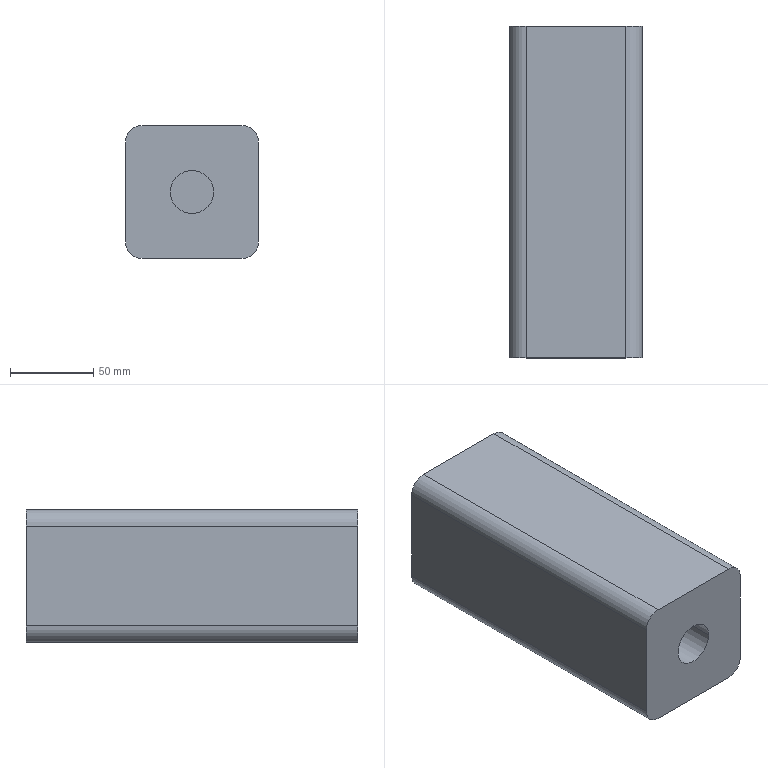Part | SolidWorks | features HoleWzd 2, Extrusion 1, Fillet 1, ICE 1 | 1 solid | 29 faces | box 80 x 199.7 x 80 mm | volume 1203112 mm3 | cylinder 14 | cone 8 | plane 7 | commonest cylinder face diameters 8.5 x8 20 x4 26 x2
STEP:
#1=CARTESIAN_POINT('',(20.,139.7,14.25));
#2=VERTEX_POINT('',#1);
#3=CARTESIAN_POINT('',(20.,139.7,5.75));
#4=VERTEX_POINT('',#3);
#5=CARTESIAN_POINT('',(20.,139.7,10.));
#6=DIRECTION('',(1.,0.,0.));
#7=DIRECTION('',(0.,0.,-1.));
#8=AXIS2_PLACEMENT_3D('',#5,#6,#7);
#9=CIRCLE('',#8,4.25);
#10=EDGE_CURVE('',#2,#4,#9,.T.);
#11=ORIENTED_EDGE('',*,*,#10,.F.);
#12=CARTESIAN_POINT('',(40.,139.7,14.25));
#13=VERTEX_POINT('',#12);
#14=CARTESIAN_POINT('',(40.,139.7,14.25));
#15=DIRECTION('',(1.,0.,0.));
#16=VECTOR('',#15,1000.);
#17=LINE('',#14,#16);
#18=EDGE_CURVE('',#2,#13,#17,.T.);
#19=ORIENTED_EDGE('',*,*,#18,.T.);
#20=CARTESIAN_POINT('',(40.,139.7,5.75));
#21=VERTEX_POINT('',#20);
#22=CARTESIAN_POINT('',(40.,139.7,10.));
#23=DIRECTION('',(1.,0.,0.));
#24=DIRECTION('',(0.,0.,-1.));
#25=AXIS2_PLACEMENT_3D('',#22,#23,#24);
#26=CIRCLE('',#25,4.25);
#27=EDGE_CURVE('',#13,#21,#26,.T.);
#28=ORIENTED_EDGE('',*,*,#27,.T.);
#29=CARTESIAN_POINT('',(40.,139.7,5.75));
#30=DIRECTION('',(1.,0.,0.));
#31=VECTOR('',#30,1000.);
#32=LINE('',#29,#31);
#33=EDGE_CURVE('',#4,#21,#32,.T.);
#34=ORIENTED_EDGE('',*,*,#33,.F.);
#35=EDGE_LOOP('',(#11,#19,#28,#34));
#36=FACE_OUTER_BOUND('',#35,.T.);
#37=CARTESIAN_POINT('',(40.,139.7,10.));
#38=DIRECTION('',(1.,0.,0.));
#39=DIRECTION('',(0.,0.,-1.));
#40=AXIS2_PLACEMENT_3D('',#37,#38,#39);
#41=CYLINDRICAL_SURFACE('',#40,4.25);
#42=ADVANCED_FACE('',(#36),#41,.F.);
#43=CARTESIAN_POINT('',(17.446,139.7,10.));
#44=VERTEX_POINT('',#43);
#45=CARTESIAN_POINT('',(20.,139.7,5.75));
#46=DIRECTION('',(0.515,0.,-0.8572));
#47=VECTOR('',#46,1000.);
#48=LINE('',#45,#47);
#49=EDGE_CURVE('',#44,#4,#48,.T.);
#50=ORIENTED_EDGE('',*,*,#49,.F.);
#51=CARTESIAN_POINT('',(20.,139.7,14.25));
#52=DIRECTION('',(0.515,0.,0.8572));
#53=VECTOR('',#52,1000.);
#54=LINE('',#51,#53);
#55=EDGE_CURVE('',#44,#2,#54,.T.);
#56=ORIENTED_EDGE('',*,*,#55,.T.);
#57=ORIENTED_EDGE('',*,*,#10,.T.);
#58=EDGE_LOOP('',(#50,#56,#57));
#59=FACE_OUTER_BOUND('',#58,.T.);
#60=CARTESIAN_POINT('',(20.,139.7,10.));
#61=DIRECTION('',(1.,0.,0.));
#62=DIRECTION('',(0.,0.,-1.));
#63=AXIS2_PLACEMENT_3D('',#60,#61,#62);
#64=CONICAL_SURFACE('',#63,4.25,1.03);
#65=ADVANCED_FACE('',(#59),#64,.F.);
#66=CARTESIAN_POINT('',(-13.,100.,10.));
#67=VERTEX_POINT('',#66);
#68=CARTESIAN_POINT('',(13.,100.,10.));
#69=VERTEX_POINT('',#68);
#70=CARTESIAN_POINT('',(0.,100.,10.));
#71=DIRECTION('',(0.,-1.,0.));
#72=DIRECTION('',(1.,0.,0.));
#73=AXIS2_PLACEMENT_3D('',#70,#71,#72);
#74=CIRCLE('',#73,13.);
#75=EDGE_CURVE('',#67,#69,#74,.T.);
#76=ORIENTED_EDGE('',*,*,#75,.F.);
#77=CARTESIAN_POINT('',(-13.,0.,10.));
#78=VERTEX_POINT('',#77);
#79=CARTESIAN_POINT('',(-13.,100.,10.));
#80=DIRECTION('',(0.,-1.,0.));
#81=VECTOR('',#80,1000.);
#82=LINE('',#79,#81);
#83=EDGE_CURVE('',#67,#78,#82,.T.);
#84=ORIENTED_EDGE('',*,*,#83,.T.);
#85=CARTESIAN_POINT('',(13.,0.,10.));
#86=VERTEX_POINT('',#85);
#87=CARTESIAN_POINT('',(0.,0.,10.));
#88=DIRECTION('',(0.,-1.,0.));
#89=DIRECTION('',(1.,0.,0.));
#90=AXIS2_PLACEMENT_3D('',#87,#88,#89);
#91=CIRCLE('',#90,13.);
#92=EDGE_CURVE('',#78,#86,#91,.T.);
#93=ORIENTED_EDGE('',*,*,#92,.T.);
#94=CARTESIAN_POINT('',(13.,100.,10.));
#95=DIRECTION('',(0.,-1.,0.));
#96=VECTOR('',#95,1000.);
#97=LINE('',#94,#96);
#98=EDGE_CURVE('',#69,#86,#97,.T.);
#99=ORIENTED_EDGE('',*,*,#98,.F.);
#100=EDGE_LOOP('',(#76,#84,#93,#99));
#101=FACE_OUTER_BOUND('',#100,.T.);
#102=CARTESIAN_POINT('',(0.,100.,10.));
#103=DIRECTION('',(0.,-1.,0.));
#104=DIRECTION('',(1.,0.,0.));
#105=AXIS2_PLACEMENT_3D('',#102,#103,#104);
#106=CYLINDRICAL_SURFACE('',#105,13.);
#107=ADVANCED_FACE('',(#101),#106,.F.);
#108=CARTESIAN_POINT('',(20.,30.,14.25));
#109=VERTEX_POINT('',#108);
#110=CARTESIAN_POINT('',(20.,30.,5.75));
#111=VERTEX_POINT('',#110);
#112=CARTESIAN_POINT('',(20.,30.,10.));
#113=DIRECTION('',(1.,0.,0.));
#114=DIRECTION('',(0.,0.,-1.));
#115=AXIS2_PLACEMENT_3D('',#112,#113,#114);
#116=CIRCLE('',#115,4.25);
#117=EDGE_CURVE('',#109,#111,#116,.T.);
#118=ORIENTED_EDGE('',*,*,#117,.F.);
#119=CARTESIAN_POINT('',(40.,30.,14.25));
#120=VERTEX_POINT('',#119);
#121=CARTESIAN_POINT('',(40.,30.,14.25));
#122=DIRECTION('',(1.,0.,0.));
#123=VECTOR('',#122,1000.);
#124=LINE('',#121,#123);
#125=EDGE_CURVE('',#109,#120,#124,.T.);
#126=ORIENTED_EDGE('',*,*,#125,.T.);
#127=CARTESIAN_POINT('',(40.,30.,5.75));
#128=VERTEX_POINT('',#127);
#129=CARTESIAN_POINT('',(40.,30.,10.));
#130=DIRECTION('',(1.,0.,0.));
#131=DIRECTION('',(0.,0.,-1.));
#132=AXIS2_PLACEMENT_3D('',#129,#130,#131);
#133=CIRCLE('',#132,4.25);
#134=EDGE_CURVE('',#120,#128,#133,.T.);
#135=ORIENTED_EDGE('',*,*,#134,.T.);
#136=CARTESIAN_POINT('',(40.,30.,5.75));
#137=DIRECTION('',(1.,0.,0.));
#138=VECTOR('',#137,1000.);
#139=LINE('',#136,#138);
#140=EDGE_CURVE('',#111,#128,#139,.T.);
#141=ORIENTED_EDGE('',*,*,#140,.F.);
#142=EDGE_LOOP('',(#118,#126,#135,#141));
#143=FACE_OUTER_BOUND('',#142,.T.);
#144=CARTESIAN_POINT('',(40.,30.,10.));
#145=DIRECTION('',(1.,0.,0.));
#146=DIRECTION('',(0.,0.,-1.));
#147=AXIS2_PLACEMENT_3D('',#144,#145,#146);
#148=CYLINDRICAL_SURFACE('',#147,4.25);
#149=ADVANCED_FACE('',(#143),#148,.F.);
#150=CARTESIAN_POINT('',(17.446,30.,10.));
#151=VERTEX_POINT('',#150);
#152=CARTESIAN_POINT('',(20.,30.,5.75));
#153=DIRECTION('',(0.515,0.,-0.8572));
#154=VECTOR('',#153,1000.);
#155=LINE('',#152,#154);
#156=EDGE_CURVE('',#151,#111,#155,.T.);
#157=ORIENTED_EDGE('',*,*,#156,.F.);
#158=CARTESIAN_POINT('',(20.,30.,14.25));
#159=DIRECTION('',(0.515,0.,0.8572));
#160=VECTOR('',#159,1000.);
#161=LINE('',#158,#160);
#162=EDGE_CURVE('',#151,#109,#161,.T.);
#163=ORIENTED_EDGE('',*,*,#162,.T.);
#164=ORIENTED_EDGE('',*,*,#117,.T.);
#165=EDGE_LOOP('',(#157,#163,#164));
#166=FACE_OUTER_BOUND('',#165,.T.);
#167=CARTESIAN_POINT('',(20.,30.,10.));
#168=DIRECTION('',(1.,0.,0.));
#169=DIRECTION('',(0.,0.,-1.));
#170=AXIS2_PLACEMENT_3D('',#167,#168,#169);
#171=CONICAL_SURFACE('',#170,4.25,1.03);
#172=ADVANCED_FACE('',(#166),#171,.F.);
#173=CARTESIAN_POINT('',(20.,179.7,14.25));
#174=VERTEX_POINT('',#173);
#175=CARTESIAN_POINT('',(20.,179.7,5.75));
#176=VERTEX_POINT('',#175);
#177=CARTESIAN_POINT('',(20.,179.7,10.));
#178=DIRECTION('',(1.,0.,0.));
#179=DIRECTION('',(0.,0.,-1.));
#180=AXIS2_PLACEMENT_3D('',#177,#178,#179);
#181=CIRCLE('',#180,4.25);
#182=EDGE_CURVE('',#174,#176,#181,.T.);
#183=ORIENTED_EDGE('',*,*,#182,.F.);
#184=CARTESIAN_POINT('',(40.,179.7,14.25));
#185=VERTEX_POINT('',#184);
#186=CARTESIAN_POINT('',(40.,179.7,14.25));
#187=DIRECTION('',(1.,0.,0.));
#188=VECTOR('',#187,1000.);
#189=LINE('',#186,#188);
#190=EDGE_CURVE('',#174,#185,#189,.T.);
#191=ORIENTED_EDGE('',*,*,#190,.T.);
#192=CARTESIAN_POINT('',(40.,179.7,5.75));
#193=VERTEX_POINT('',#192);
#194=CARTESIAN_POINT('',(40.,179.7,10.));
#195=DIRECTION('',(1.,0.,0.));
#196=DIRECTION('',(0.,0.,-1.));
#197=AXIS2_PLACEMENT_3D('',#194,#195,#196);
#198=CIRCLE('',#197,4.25);
#199=EDGE_CURVE('',#185,#193,#198,.T.);
#200=ORIENTED_EDGE('',*,*,#199,.T.);
#201=CARTESIAN_POINT('',(40.,179.7,5.75));
#202=DIRECTION('',(1.,0.,0.));
#203=VECTOR('',#202,1000.);
#204=LINE('',#201,#203);
#205=EDGE_CURVE('',#176,#193,#204,.T.);
#206=ORIENTED_EDGE('',*,*,#205,.F.);
#207=EDGE_LOOP('',(#183,#191,#200,#206));
#208=FACE_OUTER_BOUND('',#207,.T.);
#209=CARTESIAN_POINT('',(40.,179.7,10.));
#210=DIRECTION('',(1.,0.,0.));
#211=DIRECTION('',(0.,0.,-1.));
#212=AXIS2_PLACEMENT_3D('',#209,#210,#211);
#213=CYLINDRICAL_SURFACE('',#212,4.25);
#214=ADVANCED_FACE('',(#208),#213,.F.);
#215=CARTESIAN_POINT('',(17.446,179.7,10.));
#216=VERTEX_POINT('',#215);
#217=CARTESIAN_POINT('',(20.,179.7,5.75));
#218=DIRECTION('',(0.515,0.,-0.8572));
#219=VECTOR('',#218,1000.);
#220=LINE('',#217,#219);
#221=EDGE_CURVE('',#216,#176,#220,.T.);
#222=ORIENTED_EDGE('',*,*,#221,.F.);
#223=CARTESIAN_POINT('',(20.,179.7,14.25));
#224=DIRECTION('',(0.515,0.,0.8572));
#225=VECTOR('',#224,1000.);
#226=LINE('',#223,#225);
#227=EDGE_CURVE('',#216,#174,#226,.T.);
#228=ORIENTED_EDGE('',*,*,#227,.T.);
#229=ORIENTED_EDGE('',*,*,#182,.T.);
#230=EDGE_LOOP('',(#222,#228,#229));
#231=FACE_OUTER_BOUND('',#230,.T.);
#232=CARTESIAN_POINT('',(20.,179.7,10.));
#233=DIRECTION('',(1.,0.,0.));
#234=DIRECTION('',(0.,0.,-1.));
#235=AXIS2_PLACEMENT_3D('',#232,#233,#234);
#236=CONICAL_SURFACE('',#235,4.25,1.03);
#237=ADVANCED_FACE('',(#231),#236,.F.);
#238=CARTESIAN_POINT('',(20.,70.,14.25));
#239=VERTEX_POINT('',#238);
#240=CARTESIAN_POINT('',(20.,70.,5.75));
#241=VERTEX_POINT('',#240);
#242=CARTESIAN_POINT('',(20.,70.,10.));
#243=DIRECTION('',(1.,0.,0.));
#244=DIRECTION('',(0.,0.,-1.));
#245=AXIS2_PLACEMENT_3D('',#242,#243,#244);
#246=CIRCLE('',#245,4.25);
#247=EDGE_CURVE('',#239,#241,#246,.T.);
#248=ORIENTED_EDGE('',*,*,#247,.F.);
#249=CARTESIAN_POINT('',(40.,70.,14.25));
#250=VERTEX_POINT('',#249);
#251=CARTESIAN_POINT('',(40.,70.,14.25));
#252=DIRECTION('',(1.,0.,0.));
#253=VECTOR('',#252,1000.);
#254=LINE('',#251,#253);
#255=EDGE_CURVE('',#239,#250,#254,.T.);
#256=ORIENTED_EDGE('',*,*,#255,.T.);
#257=CARTESIAN_POINT('',(40.,70.,5.75));
#258=VERTEX_POINT('',#257);
#259=CARTESIAN_POINT('',(40.,70.,10.));
#260=DIRECTION('',(1.,0.,0.));
#261=DIRECTION('',(0.,0.,-1.));
#262=AXIS2_PLACEMENT_3D('',#259,#260,#261);
#263=CIRCLE('',#262,4.25);
#264=EDGE_CURVE('',#250,#258,#263,.T.);
#265=ORIENTED_EDGE('',*,*,#264,.T.);
#266=CARTESIAN_POINT('',(40.,70.,5.75));
#267=DIRECTION('',(1.,0.,0.));
#268=VECTOR('',#267,1000.);
#269=LINE('',#266,#268);
#270=EDGE_CURVE('',#241,#258,#269,.T.);
#271=ORIENTED_EDGE('',*,*,#270,.F.);
#272=EDGE_LOOP('',(#248,#256,#265,#271));
#273=FACE_OUTER_BOUND('',#272,.T.);
#274=CARTESIAN_POINT('',(40.,70.,10.));
#275=DIRECTION('',(1.,0.,0.));
#276=DIRECTION('',(0.,0.,-1.));
#277=AXIS2_PLACEMENT_3D('',#274,#275,#276);
#278=CYLINDRICAL_SURFACE('',#277,4.25);
#279=ADVANCED_FACE('',(#273),#278,.F.);
#280=CARTESIAN_POINT('',(17.446,70.,10.));
#281=VERTEX_POINT('',#280);
#282=CARTESIAN_POINT('',(20.,70.,5.75));
#283=DIRECTION('',(0.515,0.,-0.8572));
#284=VECTOR('',#283,1000.);
#285=LINE('',#282,#284);
#286=EDGE_CURVE('',#281,#241,#285,.T.);
#287=ORIENTED_EDGE('',*,*,#286,.F.);
#288=CARTESIAN_POINT('',(20.,70.,14.25));
#289=DIRECTION('',(0.515,0.,0.8572));
#290=VECTOR('',#289,1000.);
#291=LINE('',#288,#290);
#292=EDGE_CURVE('',#281,#239,#291,.T.);
#293=ORIENTED_EDGE('',*,*,#292,.T.);
#294=ORIENTED_EDGE('',*,*,#247,.T.);
#295=EDGE_LOOP('',(#287,#293,#294));
#296=FACE_OUTER_BOUND('',#295,.T.);
#297=CARTESIAN_POINT('',(20.,70.,10.));
#298=DIRECTION('',(1.,0.,0.));
#299=DIRECTION('',(0.,0.,-1.));
#300=AXIS2_PLACEMENT_3D('',#297,#298,#299);
#301=CONICAL_SURFACE('',#300,4.25,1.03);
#302=ADVANCED_FACE('',(#296),#301,.F.);
#303=CARTESIAN_POINT('',(40.,139.7,10.));
#304=DIRECTION('',(1.,0.,0.));
#305=DIRECTION('',(0.,0.,-1.));
#306=AXIS2_PLACEMENT_3D('',#303,#304,#305);
#307=CIRCLE('',#306,4.25);
#308=EDGE_CURVE('',#21,#13,#307,.T.);
#309=ORIENTED_EDGE('',*,*,#308,.F.);
#310=ORIENTED_EDGE('',*,*,#27,.F.);
#311=EDGE_LOOP('',(#309,#310));
#312=FACE_BOUND('',#311,.T.);
#313=CARTESIAN_POINT('',(40.,30.,10.));
#314=DIRECTION('',(1.,0.,0.));
#315=DIRECTION('',(0.,0.,-1.));
#316=AXIS2_PLACEMENT_3D('',#313,#314,#315);
#317=CIRCLE('',#316,4.25);
#318=EDGE_CURVE('',#128,#120,#317,.T.);
#319=ORIENTED_EDGE('',*,*,#318,.F.);
#320=ORIENTED_EDGE('',*,*,#134,.F.);
#321=EDGE_LOOP('',(#319,#320));
#322=FACE_BOUND('',#321,.T.);
#323=CARTESIAN_POINT('',(40.,179.7,10.));
#324=DIRECTION('',(1.,0.,0.));
#325=DIRECTION('',(0.,0.,-1.));
#326=AXIS2_PLACEMENT_3D('',#323,#324,#325);
#327=CIRCLE('',#326,4.25);
#328=EDGE_CURVE('',#193,#185,#327,.T.);
#329=ORIENTED_EDGE('',*,*,#328,.F.);
#330=ORIENTED_EDGE('',*,*,#199,.F.);
#331=EDGE_LOOP('',(#329,#330));
#332=FACE_BOUND('',#331,.T.);
#333=CARTESIAN_POINT('',(40.,70.,10.));
#334=DIRECTION('',(1.,0.,0.));
#335=DIRECTION('',(0.,0.,-1.));
#336=AXIS2_PLACEMENT_3D('',#333,#334,#335);
#337=CIRCLE('',#336,4.25);
#338=EDGE_CURVE('',#258,#250,#337,.T.);
#339=ORIENTED_EDGE('',*,*,#338,.F.);
#340=ORIENTED_EDGE('',*,*,#264,.F.);
#341=EDGE_LOOP('',(#339,#340));
#342=FACE_BOUND('',#341,.T.);
#343=CARTESIAN_POINT('',(40.,199.7,40.));
#344=VERTEX_POINT('',#343);
#345=CARTESIAN_POINT('',(40.,199.7,-20.));
#346=VERTEX_POINT('',#345);
#347=CARTESIAN_POINT('',(40.,199.7,50.));
#348=DIRECTION('',(0.,0.,-1.));
#349=VECTOR('',#348,1000.);
#350=LINE('',#347,#349);
#351=EDGE_CURVE('',#344,#346,#350,.T.);
#352=ORIENTED_EDGE('',*,*,#351,.F.);
#353=CARTESIAN_POINT('',(40.,0.,40.));
#354=VERTEX_POINT('',#353);
#355=CARTESIAN_POINT('',(40.,0.,40.));
#356=DIRECTION('',(0.,-1.,0.));
#357=VECTOR('',#356,1000.);
#358=LINE('',#355,#357);
#359=EDGE_CURVE('',#344,#354,#358,.T.);
#360=ORIENTED_EDGE('',*,*,#359,.T.);
#361=CARTESIAN_POINT('',(40.,0.,-20.));
#362=VERTEX_POINT('',#361);
#363=CARTESIAN_POINT('',(40.,0.,50.));
#364=DIRECTION('',(0.,0.,-1.));
#365=VECTOR('',#364,1000.);
#366=LINE('',#363,#365);
#367=EDGE_CURVE('',#354,#362,#366,.T.);
#368=ORIENTED_EDGE('',*,*,#367,.T.);
#369=CARTESIAN_POINT('',(40.,199.7,-20.));
#370=DIRECTION('',(0.,1.,0.));
#371=VECTOR('',#370,1000.);
#372=LINE('',#369,#371);
#373=EDGE_CURVE('',#362,#346,#372,.T.);
#374=ORIENTED_EDGE('',*,*,#373,.T.);
#375=EDGE_LOOP('',(#352,#360,#368,#374));
#376=FACE_OUTER_BOUND('',#375,.T.);
#377=CARTESIAN_POINT('',(40.,199.7,50.));
#378=DIRECTION('',(1.,0.,0.));
#379=DIRECTION('',(0.,1.,0.));
#380=AXIS2_PLACEMENT_3D('',#377,#378,#379);
#381=PLANE('',#380);
#382=ADVANCED_FACE('',(#312,#322,#332,#342,#376),#381,.T.);
#383=CARTESIAN_POINT('',(-30.,199.7,50.));
#384=VERTEX_POINT('',#383);
#385=CARTESIAN_POINT('',(30.,199.7,50.));
#386=VERTEX_POINT('',#385);
#387=CARTESIAN_POINT('',(-40.,199.7,50.));
#388=DIRECTION('',(1.,0.,0.));
#389=VECTOR('',#388,1000.);
#390=LINE('',#387,#389);
#391=EDGE_CURVE('',#384,#386,#390,.T.);
#392=ORIENTED_EDGE('',*,*,#391,.T.);
#393=CARTESIAN_POINT('',(30.,199.7,40.));
#394=DIRECTION('',(0.,1.,0.));
#395=DIRECTION('',(0.,0.,1.));
#396=AXIS2_PLACEMENT_3D('',#393,#394,#395);
#397=CIRCLE('',#396,10.);
#398=EDGE_CURVE('',#386,#344,#397,.T.);
#399=ORIENTED_EDGE('',*,*,#398,.T.);
#400=ORIENTED_EDGE('',*,*,#351,.T.);
#401=CARTESIAN_POINT('',(30.,199.7,-30.));
#402=VERTEX_POINT('',#401);
#403=CARTESIAN_POINT('',(30.,199.7,-20.));
#404=DIRECTION('',(0.,1.,0.));
#405=DIRECTION('',(0.,0.,1.));
#406=AXIS2_PLACEMENT_3D('',#403,#404,#405);
#407=CIRCLE('',#406,10.);
#408=EDGE_CURVE('',#346,#402,#407,.T.);
#409=ORIENTED_EDGE('',*,*,#408,.T.);
#410=CARTESIAN_POINT('',(-30.,199.7,-30.));
#411=VERTEX_POINT('',#410);
#412=CARTESIAN_POINT('',(-40.,199.7,-30.));
#413=DIRECTION('',(1.,0.,0.));
#414=VECTOR('',#413,1000.);
#415=LINE('',#412,#414);
#416=EDGE_CURVE('',#411,#402,#415,.T.);
#417=ORIENTED_EDGE('',*,*,#416,.F.);
#418=CARTESIAN_POINT('',(-40.,199.7,-20.));
#419=VERTEX_POINT('',#418);
#420=CARTESIAN_POINT('',(-30.,199.7,-20.));
#421=DIRECTION('',(0.,1.,0.));
#422=DIRECTION('',(0.,0.,1.));
#423=AXIS2_PLACEMENT_3D('',#420,#421,#422);
#424=CIRCLE('',#423,10.);
#425=EDGE_CURVE('',#411,#419,#424,.T.);
#426=ORIENTED_EDGE('',*,*,#425,.T.);
#427=CARTESIAN_POINT('',(-40.,199.7,40.));
#428=VERTEX_POINT('',#427);
#429=CARTESIAN_POINT('',(-40.,199.7,50.));
#430=DIRECTION('',(0.,0.,-1.));
#431=VECTOR('',#430,1000.);
#432=LINE('',#429,#431);
#433=EDGE_CURVE('',#428,#419,#432,.T.);
#434=ORIENTED_EDGE('',*,*,#433,.F.);
#435=CARTESIAN_POINT('',(-30.,199.7,40.));
#436=DIRECTION('',(0.,1.,0.));
#437=DIRECTION('',(0.,0.,1.));
#438=AXIS2_PLACEMENT_3D('',#435,#436,#437);
#439=CIRCLE('',#438,10.);
#440=EDGE_CURVE('',#428,#384,#439,.T.);
#441=ORIENTED_EDGE('',*,*,#440,.T.);
#442=EDGE_LOOP('',(#392,#399,#400,#409,#417,#426,#434,#441));
#443=FACE_OUTER_BOUND('',#442,.T.);
#444=CARTESIAN_POINT('',(-40.,199.7,50.));
#445=DIRECTION('',(0.,1.,0.));
#446=DIRECTION('',(0.,0.,1.));
#447=AXIS2_PLACEMENT_3D('',#444,#445,#446);
#448=PLANE('',#447);
#449=ADVANCED_FACE('',(#443),#448,.T.);
#450=CARTESIAN_POINT('',(-40.,0.,40.));
#451=VERTEX_POINT('',#450);
#452=CARTESIAN_POINT('',(-40.,0.,-20.));
#453=VERTEX_POINT('',#452);
#454=CARTESIAN_POINT('',(-40.,0.,50.));
#455=DIRECTION('',(0.,0.,-1.));
#456=VECTOR('',#455,1000.);
#457=LINE('',#454,#456);
#458=EDGE_CURVE('',#451,#453,#457,.T.);
#459=ORIENTED_EDGE('',*,*,#458,.F.);
#460=CARTESIAN_POINT('',(-40.,199.7,40.));
#461=DIRECTION('',(0.,1.,0.));
#462=VECTOR('',#461,1000.);
#463=LINE('',#460,#462);
#464=EDGE_CURVE('',#451,#428,#463,.T.);
#465=ORIENTED_EDGE('',*,*,#464,.T.);
#466=ORIENTED_EDGE('',*,*,#433,.T.);
#467=CARTESIAN_POINT('',(-40.,0.,-20.));
#468=DIRECTION('',(0.,-1.,0.));
#469=VECTOR('',#468,1000.);
#470=LINE('',#467,#469);
#471=EDGE_CURVE('',#419,#453,#470,.T.);
#472=ORIENTED_EDGE('',*,*,#471,.T.);
#473=EDGE_LOOP('',(#459,#465,#466,#472));
#474=FACE_OUTER_BOUND('',#473,.T.);
#475=CARTESIAN_POINT('',(-40.,0.,50.));
#476=DIRECTION('',(-1.,0.,0.));
#477=DIRECTION('',(0.,0.,1.));
#478=AXIS2_PLACEMENT_3D('',#475,#476,#477);
#479=PLANE('',#478);
#480=ADVANCED_FACE('',(#474),#479,.T.);
#481=CARTESIAN_POINT('',(0.,0.,10.));
#482=DIRECTION('',(0.,-1.,0.));
#483=DIRECTION('',(1.,0.,0.));
#484=AXIS2_PLACEMENT_3D('',#481,#482,#483);
#485=CIRCLE('',#484,13.);
#486=EDGE_CURVE('',#86,#78,#485,.T.);
#487=ORIENTED_EDGE('',*,*,#486,.F.);
#488=ORIENTED_EDGE('',*,*,#92,.F.);
#489=EDGE_LOOP('',(#487,#488));
#490=FACE_BOUND('',#489,.T.);
#491=ORIENTED_EDGE('',*,*,#367,.F.);
#492=CARTESIAN_POINT('',(30.,0.,50.));
#493=VERTEX_POINT('',#492);
#494=CARTESIAN_POINT('',(30.,0.,40.));
#495=DIRECTION('',(0.,-1.,0.));
#496=DIRECTION('',(1.,0.,0.));
#497=AXIS2_PLACEMENT_3D('',#494,#495,#496);
#498=CIRCLE('',#497,10.);
#499=EDGE_CURVE('',#354,#493,#498,.T.);
#500=ORIENTED_EDGE('',*,*,#499,.T.);
#501=CARTESIAN_POINT('',(-30.,0.,50.));
#502=VERTEX_POINT('',#501);
#503=CARTESIAN_POINT('',(40.,0.,50.));
#504=DIRECTION('',(-1.,0.,0.));
#505=VECTOR('',#504,1000.);
#506=LINE('',#503,#505);
#507=EDGE_CURVE('',#493,#502,#506,.T.);
#508=ORIENTED_EDGE('',*,*,#507,.T.);
#509=CARTESIAN_POINT('',(-30.,0.,40.));
#510=DIRECTION('',(0.,-1.,0.));
#511=DIRECTION('',(1.,0.,0.));
#512=AXIS2_PLACEMENT_3D('',#509,#510,#511);
#513=CIRCLE('',#512,10.);
#514=EDGE_CURVE('',#502,#451,#513,.T.);
#515=ORIENTED_EDGE('',*,*,#514,.T.);
#516=ORIENTED_EDGE('',*,*,#458,.T.);
#517=CARTESIAN_POINT('',(-30.,0.,-30.));
#518=VERTEX_POINT('',#517);
#519=CARTESIAN_POINT('',(-30.,0.,-20.));
#520=DIRECTION('',(0.,-1.,0.));
#521=DIRECTION('',(1.,0.,0.));
#522=AXIS2_PLACEMENT_3D('',#519,#520,#521);
#523=CIRCLE('',#522,10.);
#524=EDGE_CURVE('',#453,#518,#523,.T.);
#525=ORIENTED_EDGE('',*,*,#524,.T.);
#526=CARTESIAN_POINT('',(30.,0.,-30.));
#527=VERTEX_POINT('',#526);
#528=CARTESIAN_POINT('',(40.,0.,-30.));
#529=DIRECTION('',(-1.,0.,0.));
#530=VECTOR('',#529,1000.);
#531=LINE('',#528,#530);
#532=EDGE_CURVE('',#527,#518,#531,.T.);
#533=ORIENTED_EDGE('',*,*,#532,.F.);
#534=CARTESIAN_POINT('',(30.,0.,-20.));
#535=DIRECTION('',(0.,-1.,0.));
#536=DIRECTION('',(1.,0.,0.));
#537=AXIS2_PLACEMENT_3D('',#534,#535,#536);
#538=CIRCLE('',#537,10.);
#539=EDGE_CURVE('',#527,#362,#538,.T.);
#540=ORIENTED_EDGE('',*,*,#539,.T.);
#541=EDGE_LOOP('',(#491,#500,#508,#515,#516,#525,#533,#540));
#542=FACE_OUTER_BOUND('',#541,.T.);
#543=CARTESIAN_POINT('',(40.,0.,50.));
#544=DIRECTION('',(0.,-1.,0.));
#545=DIRECTION('',(1.,0.,0.));
#546=AXIS2_PLACEMENT_3D('',#543,#544,#545);
#547=PLANE('',#546);
#548=ADVANCED_FACE('',(#490,#542),#547,.T.);
#549=ORIENTED_EDGE('',*,*,#507,.F.);
#550=CARTESIAN_POINT('',(30.,199.7,50.));
#551=DIRECTION('',(0.,1.,0.));
#552=VECTOR('',#551,1000.);
#553=LINE('',#550,#552);
#554=EDGE_CURVE('',#493,#386,#553,.T.);
#555=ORIENTED_EDGE('',*,*,#554,.T.);
#556=ORIENTED_EDGE('',*,*,#391,.F.);
#557=CARTESIAN_POINT('',(-30.,0.,50.));
#558=DIRECTION('',(0.,-1.,0.));
#559=VECTOR('',#558,1000.);
#560=LINE('',#557,#559);
#561=EDGE_CURVE('',#384,#502,#560,.T.);
#562=ORIENTED_EDGE('',*,*,#561,.T.);
#563=EDGE_LOOP('',(#549,#555,#556,#562));
#564=FACE_OUTER_BOUND('',#563,.T.);
#565=CARTESIAN_POINT('',(0.,0.,50.));
#566=DIRECTION('',(0.,0.,-1.));
#567=DIRECTION('',(-1.,0.,0.));
#568=AXIS2_PLACEMENT_3D('',#565,#566,#567);
#569=PLANE('',#568);
#570=ADVANCED_FACE('',(#564),#569,.F.);
#571=ORIENTED_EDGE('',*,*,#416,.T.);
#572=CARTESIAN_POINT('',(30.,0.,-30.));
#573=DIRECTION('',(0.,-1.,0.));
#574=VECTOR('',#573,1000.);
#575=LINE('',#572,#574);
#576=EDGE_CURVE('',#402,#527,#575,.T.);
#577=ORIENTED_EDGE('',*,*,#576,.T.);
#578=ORIENTED_EDGE('',*,*,#532,.T.);
#579=CARTESIAN_POINT('',(-30.,0.,-30.));
#580=DIRECTION('',(0.,1.,0.));
#581=VECTOR('',#580,1000.);
#582=LINE('',#579,#581);
#583=EDGE_CURVE('',#518,#411,#582,.T.);
#584=ORIENTED_EDGE('',*,*,#583,.T.);
#585=EDGE_LOOP('',(#571,#577,#578,#584));
#586=FACE_OUTER_BOUND('',#585,.T.);
#587=CARTESIAN_POINT('',(0.,0.,-30.));
#588=DIRECTION('',(0.,0.,-1.));
#589=DIRECTION('',(-1.,0.,0.));
#590=AXIS2_PLACEMENT_3D('',#587,#588,#589);
#591=PLANE('',#590);
#592=ADVANCED_FACE('',(#586),#591,.T.);
#593=ORIENTED_EDGE('',*,*,#292,.F.);
#594=ORIENTED_EDGE('',*,*,#286,.T.);
#595=CARTESIAN_POINT('',(20.,70.,10.));
#596=DIRECTION('',(1.,0.,0.));
#597=DIRECTION('',(0.,0.,-1.));
#598=AXIS2_PLACEMENT_3D('',#595,#596,#597);
#599=CIRCLE('',#598,4.25);
#600=EDGE_CURVE('',#241,#239,#599,.T.);
#601=ORIENTED_EDGE('',*,*,#600,.T.);
#602=EDGE_LOOP('',(#593,#594,#601));
#603=FACE_OUTER_BOUND('',#602,.T.);
#604=CARTESIAN_POINT('',(20.,70.,10.));
#605=DIRECTION('',(1.,0.,0.));
#606=DIRECTION('',(0.,0.,-1.));
#607=AXIS2_PLACEMENT_3D('',#604,#605,#606);
#608=CONICAL_SURFACE('',#607,4.25,1.03);
#609=ADVANCED_FACE('',(#603),#608,.F.);
#610=ORIENTED_EDGE('',*,*,#255,.F.);
#611=ORIENTED_EDGE('',*,*,#600,.F.);
#612=ORIENTED_EDGE('',*,*,#270,.T.);
#613=ORIENTED_EDGE('',*,*,#338,.T.);
#614=EDGE_LOOP('',(#610,#611,#612,#613));
#615=FACE_OUTER_BOUND('',#614,.T.);
#616=CARTESIAN_POINT('',(40.,70.,10.));
#617=DIRECTION('',(1.,0.,0.));
#618=DIRECTION('',(0.,0.,-1.));
#619=AXIS2_PLACEMENT_3D('',#616,#617,#618);
#620=CYLINDRICAL_SURFACE('',#619,4.25);
#621=ADVANCED_FACE('',(#615),#620,.F.);
#622=ORIENTED_EDGE('',*,*,#227,.F.);
#623=ORIENTED_EDGE('',*,*,#221,.T.);
#624=CARTESIAN_POINT('',(20.,179.7,10.));
#625=DIRECTION('',(1.,0.,0.));
#626=DIRECTION('',(0.,0.,-1.));
#627=AXIS2_PLACEMENT_3D('',#624,#625,#626);
#628=CIRCLE('',#627,4.25);
#629=EDGE_CURVE('',#176,#174,#628,.T.);
#630=ORIENTED_EDGE('',*,*,#629,.T.);
#631=EDGE_LOOP('',(#622,#623,#630));
#632=FACE_OUTER_BOUND('',#631,.T.);
#633=CARTESIAN_POINT('',(20.,179.7,10.));
#634=DIRECTION('',(1.,0.,0.));
#635=DIRECTION('',(0.,0.,-1.));
#636=AXIS2_PLACEMENT_3D('',#633,#634,#635);
#637=CONICAL_SURFACE('',#636,4.25,1.03);
#638=ADVANCED_FACE('',(#632),#637,.F.);
#639=ORIENTED_EDGE('',*,*,#190,.F.);
#640=ORIENTED_EDGE('',*,*,#629,.F.);
#641=ORIENTED_EDGE('',*,*,#205,.T.);
#642=ORIENTED_EDGE('',*,*,#328,.T.);
#643=EDGE_LOOP('',(#639,#640,#641,#642));
#644=FACE_OUTER_BOUND('',#643,.T.);
#645=CARTESIAN_POINT('',(40.,179.7,10.));
#646=DIRECTION('',(1.,0.,0.));
#647=DIRECTION('',(0.,0.,-1.));
#648=AXIS2_PLACEMENT_3D('',#645,#646,#647);
#649=CYLINDRICAL_SURFACE('',#648,4.25);
#650=ADVANCED_FACE('',(#644),#649,.F.);
#651=ORIENTED_EDGE('',*,*,#162,.F.);
#652=ORIENTED_EDGE('',*,*,#156,.T.);
#653=CARTESIAN_POINT('',(20.,30.,10.));
#654=DIRECTION('',(1.,0.,0.));
#655=DIRECTION('',(0.,0.,-1.));
#656=AXIS2_PLACEMENT_3D('',#653,#654,#655);
#657=CIRCLE('',#656,4.25);
#658=EDGE_CURVE('',#111,#109,#657,.T.);
#659=ORIENTED_EDGE('',*,*,#658,.T.);
#660=EDGE_LOOP('',(#651,#652,#659));
#661=FACE_OUTER_BOUND('',#660,.T.);
#662=CARTESIAN_POINT('',(20.,30.,10.));
#663=DIRECTION('',(1.,0.,0.));
#664=DIRECTION('',(0.,0.,-1.));
#665=AXIS2_PLACEMENT_3D('',#662,#663,#664);
#666=CONICAL_SURFACE('',#665,4.25,1.03);
#667=ADVANCED_FACE('',(#661),#666,.F.);
#668=ORIENTED_EDGE('',*,*,#125,.F.);
#669=ORIENTED_EDGE('',*,*,#658,.F.);
#670=ORIENTED_EDGE('',*,*,#140,.T.);
#671=ORIENTED_EDGE('',*,*,#318,.T.);
#672=EDGE_LOOP('',(#668,#669,#670,#671));
#673=FACE_OUTER_BOUND('',#672,.T.);
#674=CARTESIAN_POINT('',(40.,30.,10.));
#675=DIRECTION('',(1.,0.,0.));
#676=DIRECTION('',(0.,0.,-1.));
#677=AXIS2_PLACEMENT_3D('',#674,#675,#676);
#678=CYLINDRICAL_SURFACE('',#677,4.25);
#679=ADVANCED_FACE('',(#673),#678,.F.);
#680=ORIENTED_EDGE('',*,*,#398,.F.);
#681=ORIENTED_EDGE('',*,*,#554,.F.);
#682=ORIENTED_EDGE('',*,*,#499,.F.);
#683=ORIENTED_EDGE('',*,*,#359,.F.);
#684=EDGE_LOOP('',(#680,#681,#682,#683));
#685=FACE_OUTER_BOUND('',#684,.T.);
#686=CARTESIAN_POINT('',(30.,199.7,40.));
#687=DIRECTION('',(0.,1.,0.));
#688=DIRECTION('',(-1.,0.,0.));
#689=AXIS2_PLACEMENT_3D('',#686,#687,#688);
#690=CYLINDRICAL_SURFACE('',#689,10.);
#691=ADVANCED_FACE('',(#685),#690,.T.);
#692=ORIENTED_EDGE('',*,*,#514,.F.);
#693=ORIENTED_EDGE('',*,*,#561,.F.);
#694=ORIENTED_EDGE('',*,*,#440,.F.);
#695=ORIENTED_EDGE('',*,*,#464,.F.);
#696=EDGE_LOOP('',(#692,#693,#694,#695));
#697=FACE_OUTER_BOUND('',#696,.T.);
#698=CARTESIAN_POINT('',(-30.,0.,40.));
#699=DIRECTION('',(0.,-1.,0.));
#700=DIRECTION('',(0.,0.,-1.));
#701=AXIS2_PLACEMENT_3D('',#698,#699,#700);
#702=CYLINDRICAL_SURFACE('',#701,10.);
#703=ADVANCED_FACE('',(#697),#702,.T.);
#704=ORIENTED_EDGE('',*,*,#408,.F.);
#705=ORIENTED_EDGE('',*,*,#373,.F.);
#706=ORIENTED_EDGE('',*,*,#539,.F.);
#707=ORIENTED_EDGE('',*,*,#576,.F.);
#708=EDGE_LOOP('',(#704,#705,#706,#707));
#709=FACE_OUTER_BOUND('',#708,.T.);
#710=CARTESIAN_POINT('',(30.,0.,-20.));
#711=DIRECTION('',(0.,-1.,0.));
#712=DIRECTION('',(1.,0.,0.));
#713=AXIS2_PLACEMENT_3D('',#710,#711,#712);
#714=CYLINDRICAL_SURFACE('',#713,10.);
#715=ADVANCED_FACE('',(#709),#714,.T.);
#716=ORIENTED_EDGE('',*,*,#524,.F.);
#717=ORIENTED_EDGE('',*,*,#471,.F.);
#718=ORIENTED_EDGE('',*,*,#425,.F.);
#719=ORIENTED_EDGE('',*,*,#583,.F.);
#720=EDGE_LOOP('',(#716,#717,#718,#719));
#721=FACE_OUTER_BOUND('',#720,.T.);
#722=CARTESIAN_POINT('',(-30.,0.,-20.));
#723=DIRECTION('',(0.,1.,0.));
#724=DIRECTION('',(0.,0.,1.));
#725=AXIS2_PLACEMENT_3D('',#722,#723,#724);
#726=CYLINDRICAL_SURFACE('',#725,10.);
#727=ADVANCED_FACE('',(#721),#726,.T.);
#728=ORIENTED_EDGE('',*,*,#83,.F.);
#729=CARTESIAN_POINT('',(0.,100.,10.));
#730=DIRECTION('',(0.,-1.,0.));
#731=DIRECTION('',(1.,0.,0.));
#732=AXIS2_PLACEMENT_3D('',#729,#730,#731);
#733=CIRCLE('',#732,13.);
#734=EDGE_CURVE('',#69,#67,#733,.T.);
#735=ORIENTED_EDGE('',*,*,#734,.F.);
#736=ORIENTED_EDGE('',*,*,#98,.T.);
#737=ORIENTED_EDGE('',*,*,#486,.T.);
#738=EDGE_LOOP('',(#728,#735,#736,#737));
#739=FACE_OUTER_BOUND('',#738,.T.);
#740=CARTESIAN_POINT('',(0.,100.,10.));
#741=DIRECTION('',(0.,-1.,0.));
#742=DIRECTION('',(1.,0.,0.));
#743=AXIS2_PLACEMENT_3D('',#740,#741,#742);
#744=CYLINDRICAL_SURFACE('',#743,13.);
#745=ADVANCED_FACE('',(#739),#744,.F.);
#746=ORIENTED_EDGE('',*,*,#734,.T.);
#747=ORIENTED_EDGE('',*,*,#75,.T.);
#748=EDGE_LOOP('',(#746,#747));
#749=FACE_OUTER_BOUND('',#748,.T.);
#750=CARTESIAN_POINT('',(0.,100.,10.));
#751=DIRECTION('',(0.,-1.,0.));
#752=DIRECTION('',(1.,0.,0.));
#753=AXIS2_PLACEMENT_3D('',#750,#751,#752);
#754=PLANE('',#753);
#755=ADVANCED_FACE('',(#749),#754,.T.);
#756=ORIENTED_EDGE('',*,*,#55,.F.);
#757=ORIENTED_EDGE('',*,*,#49,.T.);
#758=CARTESIAN_POINT('',(20.,139.7,10.));
#759=DIRECTION('',(1.,0.,0.));
#760=DIRECTION('',(0.,0.,-1.));
#761=AXIS2_PLACEMENT_3D('',#758,#759,#760);
#762=CIRCLE('',#761,4.25);
#763=EDGE_CURVE('',#4,#2,#762,.T.);
#764=ORIENTED_EDGE('',*,*,#763,.T.);
#765=EDGE_LOOP('',(#756,#757,#764));
#766=FACE_OUTER_BOUND('',#765,.T.);
#767=CARTESIAN_POINT('',(20.,139.7,10.));
#768=DIRECTION('',(1.,0.,0.));
#769=DIRECTION('',(0.,0.,-1.));
#770=AXIS2_PLACEMENT_3D('',#767,#768,#769);
#771=CONICAL_SURFACE('',#770,4.25,1.03);
#772=ADVANCED_FACE('',(#766),#771,.F.);
#773=ORIENTED_EDGE('',*,*,#18,.F.);
#774=ORIENTED_EDGE('',*,*,#763,.F.);
#775=ORIENTED_EDGE('',*,*,#33,.T.);
#776=ORIENTED_EDGE('',*,*,#308,.T.);
#777=EDGE_LOOP('',(#773,#774,#775,#776));
#778=FACE_OUTER_BOUND('',#777,.T.);
#779=CARTESIAN_POINT('',(40.,139.7,10.));
#780=DIRECTION('',(1.,0.,0.));
#781=DIRECTION('',(0.,0.,-1.));
#782=AXIS2_PLACEMENT_3D('',#779,#780,#781);
#783=CYLINDRICAL_SURFACE('',#782,4.25);
#784=ADVANCED_FACE('',(#778),#783,.F.);
#785=CLOSED_SHELL('',(#42,#65,#107,#149,#172,#214,#237,#279,#302,#382,#449,#480,#548,#570,#592,#609,#621,#638,#650,#667,#679,#691,#703,#715,#727,#745,#755,#772,#784));
#786=MANIFOLD_SOLID_BREP('',#785);
#787=CARTESIAN_POINT('',(0.,0.,0.));
#788=DIRECTION('',(0.,0.,1.));
#789=DIRECTION('',(1.,0.,0.));
#790=AXIS2_PLACEMENT_3D('',#787,#788,#789);
#791=(LENGTH_UNIT()NAMED_UNIT(*)SI_UNIT(.MILLI.,.METRE.));
#792=UNCERTAINTY_MEASURE_WITH_UNIT(LENGTH_MEASURE(0.00001),#791,'','');
#793=(NAMED_UNIT(*)PLANE_ANGLE_UNIT()SI_UNIT($,.RADIAN.));
#794=(NAMED_UNIT(*)SI_UNIT($,.STERADIAN.)SOLID_ANGLE_UNIT());
#795=(GEOMETRIC_REPRESENTATION_CONTEXT(3)GLOBAL_UNCERTAINTY_ASSIGNED_CONTEXT((#792))GLOBAL_UNIT_ASSIGNED_CONTEXT((#791,#793,#794))REPRESENTATION_CONTEXT('',''));
#796=ADVANCED_BREP_SHAPE_REPRESENTATION('',(#786,#790),#795);